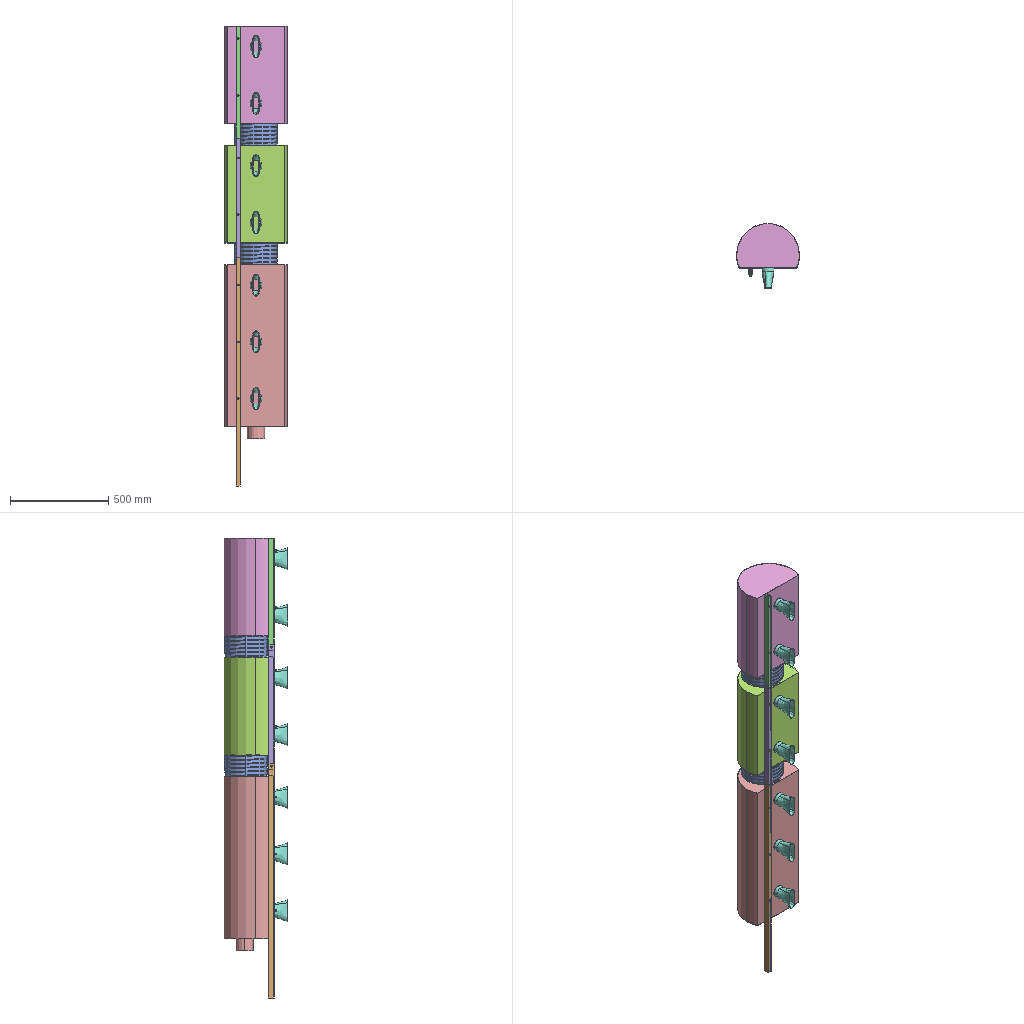Assembly | SolidWorks | 8 different items | 15 placed | box 320 x 324 x 2336 mm
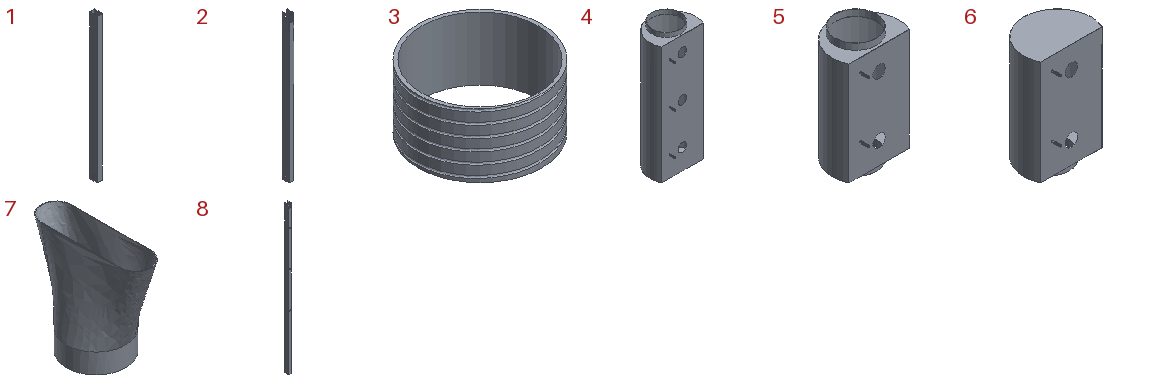Parts list (item | quantity | size | volume | features):
1 | x1 | 20 x 30 x 566 mm | 54179 mm3 | features Extrusion 1, ICE 1
2 | x1 | 22 x 30 x 631 mm | 60974 mm3 | features ICE 3, Extrusion 1, MirrorPattern 1
3 | x2 | - | 402260 mm3 | features Extrusion 1, Helix 1, SweepCut 1
4 | x1 | 320 x 266 x 914 mm | 1052652 mm3 | features ICE 8, SweepThread 3, Extrusion 1, Shell 1
5 | x1 | 320 x 266 x 556 mm | 661676 mm3 | features ICE 7, SweepThread 2, Extrusion 1, Shell 1
6 | x1 | 320 x 266 x 526 mm | 676620 mm3 | features ICE 6, SweepThread 2, Extrusion 1, Shell 1
7 | x7 | 60.001 x 111.2 x 100 mm | 12348 mm3 | features Blend 1, Extrusion 1, Shell 1
8 | x1 | 22 x 30 x 1189 mm | 114398 mm3 | features ICE 4, Extrusion 1, MirrorPattern 1
Mates (type | each side: item.copy, entity, surface, feature):
Concentric | 4.1 face cylinder Boss-Extrude7 | 3.1 face cylinder Boss-Extrude1
Coincident | 4.1 face plane Boss-Extrude1 | 3.1 face plane Boss-Extrude1
Concentric | 3.1 face cylinder Boss-Extrude1 | 5.1 face cylinder Boss-Extrude7
Coincident | 3.1 face plane Boss-Extrude1 | 5.1 face plane Boss-Extrude1
Parallel | 4.1 face plane Boss-Extrude1 | 5.1 face plane Boss-Extrude1
Concentric | 5.1 face cylinder Boss-Extrude8 | 3.2 face cylinder Boss-Extrude1
Coincident | 5.1 face plane Boss-Extrude1 | 3.2 face plane Boss-Extrude1
Concentric | 6.1 face cylinder Boss-Extrude7 | 3.2 edge
Coincident | 6.1 face plane Boss-Extrude1 | 3.2 face plane Boss-Extrude1
Parallel | 5.1 face plane Boss-Extrude1 | 6.1 face plane Boss-Extrude1
Coincident | 4.1 face plane Boss-Extrude1 | 7.1 face plane Boss-Extrude1
Concentric | 4.1 face cylinder Cut-Extrude2 | 7.1 face cylinder Shell1
Parallel | 7.1 select_type:24 | assembly select_type:10
Concentric | 5.1 face cylinder Cut-Extrude2 | 7.2 face cylinder Shell1
Coincident | 5.1 face plane Boss-Extrude1 | 7.2 face plane Boss-Extrude1
Parallel | 7.2 select_type:24 | assembly select_type:10
Concentric | 6.1 face cylinder Cut-Extrude2 | 7.3 face cylinder Shell1
Coincident | 6.1 face plane Boss-Extrude1 | 7.3 face plane Boss-Extrude1
Parallel | 7.3 select_type:24 | assembly select_type:10
Concentric | 4.1 face cylinder Boss-Extrude6 | 8.1 face cylinder Cut-Extrude2 | 2 times
Coincident | 4.1 face plane Boss-Extrude1 | 8.1 face plane Boss-Extrude1
Concentric | 8.1 face cylinder Cut-Extrude1 | 2.1 face cylinder Cut-Extrude2
Coincident | 8.1 face plane Mirror2 | 2.1 face plane Boss-Extrude1
Coincident | 5.1 face plane Boss-Extrude1 | 2.1 face plane Boss-Extrude1
Concentric | 2.1 face cylinder Cut-Extrude1 | 1.1 face cylinder Cut-Extrude1
Coincident | 2.1 face plane Mirror2 | 1.1 face plane Boss-Extrude1
Coincident | 6.1 face plane Boss-Extrude1 | 1.1 face plane Boss-Extrude1